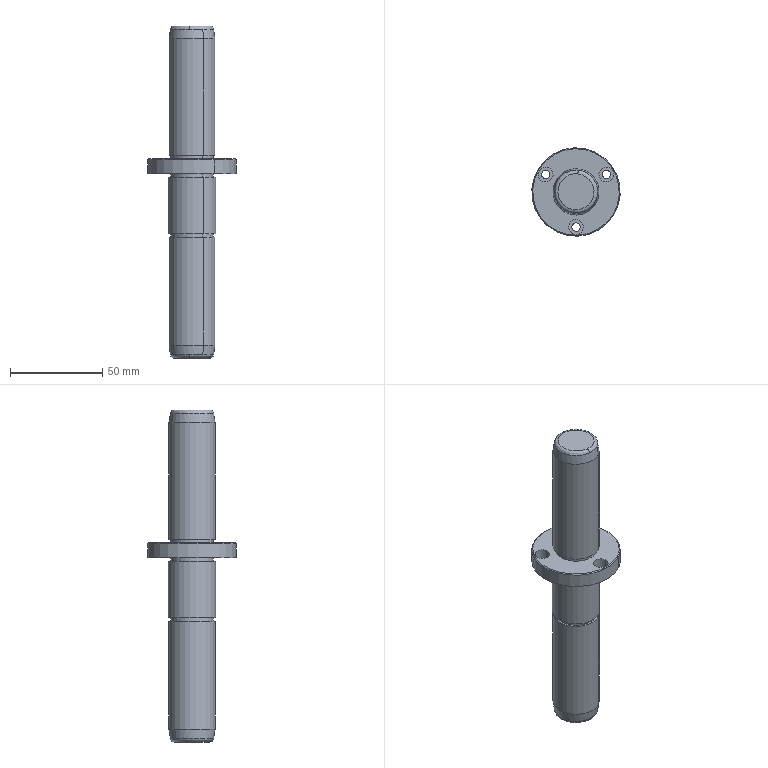Part | 1 solid | 47 faces | box 48 x 48 x 180 mm | volume 98042 mm3 | cylinder 26 | plane 11 | cone 6 | torus 4 | commonest cylinder face diameters 4.5 x6 8 x6 23 x6 25 x4 26 x2 48 x2